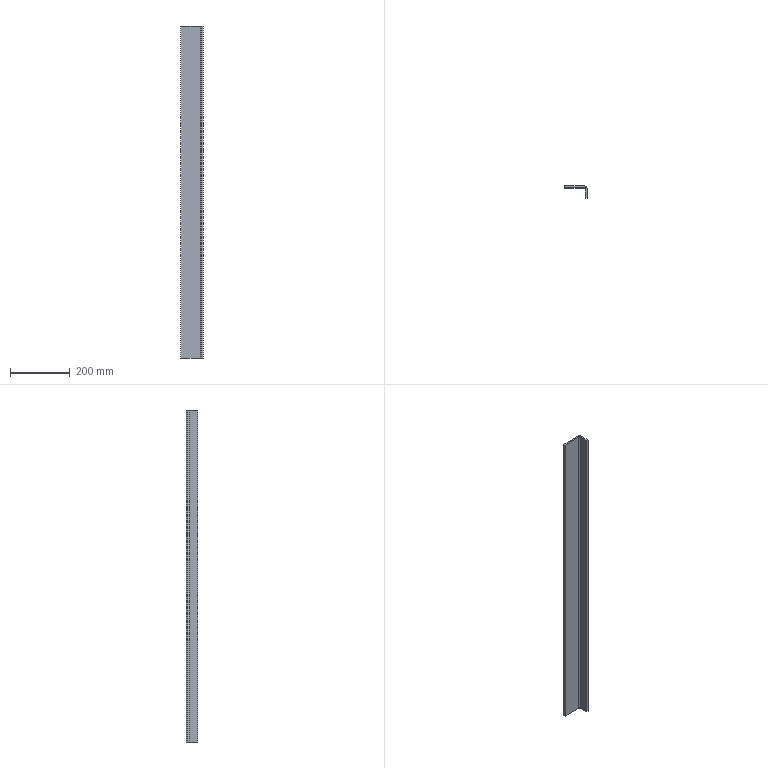Part | SolidWorks | features Extrusion 1 | 1 solid | 10 faces | box 75 x 40 x 1110 mm | volume 705931 mm3 | plane 8 | cylinder 2 | commonest cylinder face diameters 8 x1 20 x1
STEP:
#1=CARTESIAN_POINT('',(75.,-10.,0.));
#2=VERTEX_POINT('',#1);
#3=CARTESIAN_POINT('',(75.,-40.,0.));
#4=VERTEX_POINT('',#3);
#5=CARTESIAN_POINT('',(75.,-10.,0.));
#6=DIRECTION('',(0.,-1.,0.));
#7=VECTOR('',#6,1000.);
#8=LINE('',#5,#7);
#9=EDGE_CURVE('',#2,#4,#8,.T.);
#10=ORIENTED_EDGE('',*,*,#9,.F.);
#11=CARTESIAN_POINT('',(75.,-10.,1110.));
#12=VERTEX_POINT('',#11);
#13=CARTESIAN_POINT('',(75.,-10.,1110.));
#14=DIRECTION('',(0.,0.,-1.));
#15=VECTOR('',#14,1000.);
#16=LINE('',#13,#15);
#17=EDGE_CURVE('',#12,#2,#16,.T.);
#18=ORIENTED_EDGE('',*,*,#17,.F.);
#19=CARTESIAN_POINT('',(75.,-40.,1110.));
#20=VERTEX_POINT('',#19);
#21=CARTESIAN_POINT('',(75.,-10.,1110.));
#22=DIRECTION('',(0.,-1.,0.));
#23=VECTOR('',#22,1000.);
#24=LINE('',#21,#23);
#25=EDGE_CURVE('',#12,#20,#24,.T.);
#26=ORIENTED_EDGE('',*,*,#25,.T.);
#27=CARTESIAN_POINT('',(75.,-40.,1110.));
#28=DIRECTION('',(0.,0.,-1.));
#29=VECTOR('',#28,1000.);
#30=LINE('',#27,#29);
#31=EDGE_CURVE('',#20,#4,#30,.T.);
#32=ORIENTED_EDGE('',*,*,#31,.T.);
#33=EDGE_LOOP('',(#10,#18,#26,#32));
#34=FACE_OUTER_BOUND('',#33,.T.);
#35=CARTESIAN_POINT('',(75.,-10.,1110.));
#36=DIRECTION('',(1.,0.,0.));
#37=DIRECTION('',(0.,0.,-1.));
#38=AXIS2_PLACEMENT_3D('',#35,#36,#37);
#39=PLANE('',#38);
#40=ADVANCED_FACE('',(#34),#39,.T.);
#41=CARTESIAN_POINT('',(65.,0.,0.));
#42=VERTEX_POINT('',#41);
#43=CARTESIAN_POINT('',(65.,-10.,0.));
#44=DIRECTION('',(0.,0.,-1.));
#45=DIRECTION('',(-1.,0.,0.));
#46=AXIS2_PLACEMENT_3D('',#43,#44,#45);
#47=CIRCLE('',#46,10.);
#48=EDGE_CURVE('',#42,#2,#47,.T.);
#49=ORIENTED_EDGE('',*,*,#48,.F.);
#50=CARTESIAN_POINT('',(65.,0.,1110.));
#51=VERTEX_POINT('',#50);
#52=CARTESIAN_POINT('',(65.,0.,1110.));
#53=DIRECTION('',(0.,0.,-1.));
#54=VECTOR('',#53,1000.);
#55=LINE('',#52,#54);
#56=EDGE_CURVE('',#51,#42,#55,.T.);
#57=ORIENTED_EDGE('',*,*,#56,.F.);
#58=CARTESIAN_POINT('',(65.,-10.,1110.));
#59=DIRECTION('',(0.,0.,-1.));
#60=DIRECTION('',(-1.,0.,0.));
#61=AXIS2_PLACEMENT_3D('',#58,#59,#60);
#62=CIRCLE('',#61,10.);
#63=EDGE_CURVE('',#51,#12,#62,.T.);
#64=ORIENTED_EDGE('',*,*,#63,.T.);
#65=ORIENTED_EDGE('',*,*,#17,.T.);
#66=EDGE_LOOP('',(#49,#57,#64,#65));
#67=FACE_OUTER_BOUND('',#66,.T.);
#68=CARTESIAN_POINT('',(65.,-10.,1110.));
#69=DIRECTION('',(0.,0.,-1.));
#70=DIRECTION('',(-1.,0.,0.));
#71=AXIS2_PLACEMENT_3D('',#68,#69,#70);
#72=CYLINDRICAL_SURFACE('',#71,10.);
#73=ADVANCED_FACE('',(#67),#72,.T.);
#74=CARTESIAN_POINT('',(0.,0.,0.));
#75=VERTEX_POINT('',#74);
#76=CARTESIAN_POINT('',(0.,0.,0.));
#77=DIRECTION('',(1.,0.,0.));
#78=VECTOR('',#77,1000.);
#79=LINE('',#76,#78);
#80=EDGE_CURVE('',#75,#42,#79,.T.);
#81=ORIENTED_EDGE('',*,*,#80,.F.);
#82=CARTESIAN_POINT('',(0.,0.,1110.));
#83=VERTEX_POINT('',#82);
#84=CARTESIAN_POINT('',(0.,0.,1110.));
#85=DIRECTION('',(0.,0.,-1.));
#86=VECTOR('',#85,1000.);
#87=LINE('',#84,#86);
#88=EDGE_CURVE('',#83,#75,#87,.T.);
#89=ORIENTED_EDGE('',*,*,#88,.F.);
#90=CARTESIAN_POINT('',(0.,0.,1110.));
#91=DIRECTION('',(1.,0.,0.));
#92=VECTOR('',#91,1000.);
#93=LINE('',#90,#92);
#94=EDGE_CURVE('',#83,#51,#93,.T.);
#95=ORIENTED_EDGE('',*,*,#94,.T.);
#96=ORIENTED_EDGE('',*,*,#56,.T.);
#97=EDGE_LOOP('',(#81,#89,#95,#96));
#98=FACE_OUTER_BOUND('',#97,.T.);
#99=CARTESIAN_POINT('',(0.,0.,1110.));
#100=DIRECTION('',(0.,1.,0.));
#101=DIRECTION('',(0.,0.,1.));
#102=AXIS2_PLACEMENT_3D('',#99,#100,#101);
#103=PLANE('',#102);
#104=ADVANCED_FACE('',(#98),#103,.T.);
#105=CARTESIAN_POINT('',(0.,-6.,0.));
#106=VERTEX_POINT('',#105);
#107=CARTESIAN_POINT('',(0.,0.,0.));
#108=DIRECTION('',(0.,-1.,0.));
#109=VECTOR('',#108,1000.);
#110=LINE('',#107,#109);
#111=EDGE_CURVE('',#75,#106,#110,.T.);
#112=ORIENTED_EDGE('',*,*,#111,.T.);
#113=CARTESIAN_POINT('',(0.,-6.,1110.));
#114=VERTEX_POINT('',#113);
#115=CARTESIAN_POINT('',(0.,-6.,1110.));
#116=DIRECTION('',(0.,0.,-1.));
#117=VECTOR('',#116,1000.);
#118=LINE('',#115,#117);
#119=EDGE_CURVE('',#114,#106,#118,.T.);
#120=ORIENTED_EDGE('',*,*,#119,.F.);
#121=CARTESIAN_POINT('',(0.,0.,1110.));
#122=DIRECTION('',(0.,-1.,0.));
#123=VECTOR('',#122,1000.);
#124=LINE('',#121,#123);
#125=EDGE_CURVE('',#83,#114,#124,.T.);
#126=ORIENTED_EDGE('',*,*,#125,.F.);
#127=ORIENTED_EDGE('',*,*,#88,.T.);
#128=EDGE_LOOP('',(#112,#120,#126,#127));
#129=FACE_OUTER_BOUND('',#128,.T.);
#130=CARTESIAN_POINT('',(0.,0.,1110.));
#131=DIRECTION('',(1.,0.,0.));
#132=DIRECTION('',(0.,0.,-1.));
#133=AXIS2_PLACEMENT_3D('',#130,#131,#132);
#134=PLANE('',#133);
#135=ADVANCED_FACE('',(#129),#134,.F.);
#136=CARTESIAN_POINT('',(65.,-6.,0.));
#137=VERTEX_POINT('',#136);
#138=CARTESIAN_POINT('',(0.,-6.,0.));
#139=DIRECTION('',(1.,0.,0.));
#140=VECTOR('',#139,1000.);
#141=LINE('',#138,#140);
#142=EDGE_CURVE('',#106,#137,#141,.T.);
#143=ORIENTED_EDGE('',*,*,#142,.T.);
#144=CARTESIAN_POINT('',(65.,-6.,1110.));
#145=VERTEX_POINT('',#144);
#146=CARTESIAN_POINT('',(65.,-6.,1110.));
#147=DIRECTION('',(0.,0.,-1.));
#148=VECTOR('',#147,1000.);
#149=LINE('',#146,#148);
#150=EDGE_CURVE('',#145,#137,#149,.T.);
#151=ORIENTED_EDGE('',*,*,#150,.F.);
#152=CARTESIAN_POINT('',(0.,-6.,1110.));
#153=DIRECTION('',(1.,0.,0.));
#154=VECTOR('',#153,1000.);
#155=LINE('',#152,#154);
#156=EDGE_CURVE('',#114,#145,#155,.T.);
#157=ORIENTED_EDGE('',*,*,#156,.F.);
#158=ORIENTED_EDGE('',*,*,#119,.T.);
#159=EDGE_LOOP('',(#143,#151,#157,#158));
#160=FACE_OUTER_BOUND('',#159,.T.);
#161=CARTESIAN_POINT('',(0.,-6.,1110.));
#162=DIRECTION('',(0.,1.,0.));
#163=DIRECTION('',(0.,0.,1.));
#164=AXIS2_PLACEMENT_3D('',#161,#162,#163);
#165=PLANE('',#164);
#166=ADVANCED_FACE('',(#160),#165,.F.);
#167=CARTESIAN_POINT('',(69.,-10.,0.));
#168=VERTEX_POINT('',#167);
#169=CARTESIAN_POINT('',(65.,-10.,0.));
#170=DIRECTION('',(0.,0.,-1.));
#171=DIRECTION('',(-1.,0.,0.));
#172=AXIS2_PLACEMENT_3D('',#169,#170,#171);
#173=CIRCLE('',#172,4.);
#174=EDGE_CURVE('',#137,#168,#173,.T.);
#175=ORIENTED_EDGE('',*,*,#174,.T.);
#176=CARTESIAN_POINT('',(69.,-10.,1110.));
#177=VERTEX_POINT('',#176);
#178=CARTESIAN_POINT('',(69.,-10.,1110.));
#179=DIRECTION('',(0.,0.,-1.));
#180=VECTOR('',#179,1000.);
#181=LINE('',#178,#180);
#182=EDGE_CURVE('',#177,#168,#181,.T.);
#183=ORIENTED_EDGE('',*,*,#182,.F.);
#184=CARTESIAN_POINT('',(65.,-10.,1110.));
#185=DIRECTION('',(0.,0.,-1.));
#186=DIRECTION('',(-1.,0.,0.));
#187=AXIS2_PLACEMENT_3D('',#184,#185,#186);
#188=CIRCLE('',#187,4.);
#189=EDGE_CURVE('',#145,#177,#188,.T.);
#190=ORIENTED_EDGE('',*,*,#189,.F.);
#191=ORIENTED_EDGE('',*,*,#150,.T.);
#192=EDGE_LOOP('',(#175,#183,#190,#191));
#193=FACE_OUTER_BOUND('',#192,.T.);
#194=CARTESIAN_POINT('',(65.,-10.,1110.));
#195=DIRECTION('',(0.,0.,-1.));
#196=DIRECTION('',(-1.,0.,0.));
#197=AXIS2_PLACEMENT_3D('',#194,#195,#196);
#198=CYLINDRICAL_SURFACE('',#197,4.);
#199=ADVANCED_FACE('',(#193),#198,.F.);
#200=CARTESIAN_POINT('',(69.,-40.,0.));
#201=VERTEX_POINT('',#200);
#202=CARTESIAN_POINT('',(69.,-10.,0.));
#203=DIRECTION('',(0.,-1.,0.));
#204=VECTOR('',#203,1000.);
#205=LINE('',#202,#204);
#206=EDGE_CURVE('',#168,#201,#205,.T.);
#207=ORIENTED_EDGE('',*,*,#206,.T.);
#208=CARTESIAN_POINT('',(69.,-40.,1110.));
#209=VERTEX_POINT('',#208);
#210=CARTESIAN_POINT('',(69.,-40.,1110.));
#211=DIRECTION('',(0.,0.,-1.));
#212=VECTOR('',#211,1000.);
#213=LINE('',#210,#212);
#214=EDGE_CURVE('',#209,#201,#213,.T.);
#215=ORIENTED_EDGE('',*,*,#214,.F.);
#216=CARTESIAN_POINT('',(69.,-10.,1110.));
#217=DIRECTION('',(0.,-1.,0.));
#218=VECTOR('',#217,1000.);
#219=LINE('',#216,#218);
#220=EDGE_CURVE('',#177,#209,#219,.T.);
#221=ORIENTED_EDGE('',*,*,#220,.F.);
#222=ORIENTED_EDGE('',*,*,#182,.T.);
#223=EDGE_LOOP('',(#207,#215,#221,#222));
#224=FACE_OUTER_BOUND('',#223,.T.);
#225=CARTESIAN_POINT('',(69.,-10.,1110.));
#226=DIRECTION('',(1.,0.,0.));
#227=DIRECTION('',(0.,1.,0.));
#228=AXIS2_PLACEMENT_3D('',#225,#226,#227);
#229=PLANE('',#228);
#230=ADVANCED_FACE('',(#224),#229,.F.);
#231=CARTESIAN_POINT('',(75.,-40.,0.));
#232=DIRECTION('',(-1.,0.,0.));
#233=VECTOR('',#232,1000.);
#234=LINE('',#231,#233);
#235=EDGE_CURVE('',#4,#201,#234,.T.);
#236=ORIENTED_EDGE('',*,*,#235,.F.);
#237=ORIENTED_EDGE('',*,*,#31,.F.);
#238=CARTESIAN_POINT('',(75.,-40.,1110.));
#239=DIRECTION('',(-1.,0.,0.));
#240=VECTOR('',#239,1000.);
#241=LINE('',#238,#240);
#242=EDGE_CURVE('',#20,#209,#241,.T.);
#243=ORIENTED_EDGE('',*,*,#242,.T.);
#244=ORIENTED_EDGE('',*,*,#214,.T.);
#245=EDGE_LOOP('',(#236,#237,#243,#244));
#246=FACE_OUTER_BOUND('',#245,.T.);
#247=CARTESIAN_POINT('',(75.,-40.,1110.));
#248=DIRECTION('',(0.,-1.,0.));
#249=DIRECTION('',(0.,0.,-1.));
#250=AXIS2_PLACEMENT_3D('',#247,#248,#249);
#251=PLANE('',#250);
#252=ADVANCED_FACE('',(#246),#251,.T.);
#253=ORIENTED_EDGE('',*,*,#25,.F.);
#254=ORIENTED_EDGE('',*,*,#63,.F.);
#255=ORIENTED_EDGE('',*,*,#94,.F.);
#256=ORIENTED_EDGE('',*,*,#125,.T.);
#257=ORIENTED_EDGE('',*,*,#156,.T.);
#258=ORIENTED_EDGE('',*,*,#189,.T.);
#259=ORIENTED_EDGE('',*,*,#220,.T.);
#260=ORIENTED_EDGE('',*,*,#242,.F.);
#261=EDGE_LOOP('',(#253,#254,#255,#256,#257,#258,#259,#260));
#262=FACE_OUTER_BOUND('',#261,.T.);
#263=CARTESIAN_POINT('',(65.,-10.,1110.));
#264=DIRECTION('',(0.,0.,-1.));
#265=DIRECTION('',(-1.,0.,0.));
#266=AXIS2_PLACEMENT_3D('',#263,#264,#265);
#267=PLANE('',#266);
#268=ADVANCED_FACE('',(#262),#267,.F.);
#269=ORIENTED_EDGE('',*,*,#9,.T.);
#270=ORIENTED_EDGE('',*,*,#235,.T.);
#271=ORIENTED_EDGE('',*,*,#206,.F.);
#272=ORIENTED_EDGE('',*,*,#174,.F.);
#273=ORIENTED_EDGE('',*,*,#142,.F.);
#274=ORIENTED_EDGE('',*,*,#111,.F.);
#275=ORIENTED_EDGE('',*,*,#80,.T.);
#276=ORIENTED_EDGE('',*,*,#48,.T.);
#277=EDGE_LOOP('',(#269,#270,#271,#272,#273,#274,#275,#276));
#278=FACE_OUTER_BOUND('',#277,.T.);
#279=CARTESIAN_POINT('',(65.,-10.,0.));
#280=DIRECTION('',(0.,0.,-1.));
#281=DIRECTION('',(-1.,0.,0.));
#282=AXIS2_PLACEMENT_3D('',#279,#280,#281);
#283=PLANE('',#282);
#284=ADVANCED_FACE('',(#278),#283,.T.);
#285=CLOSED_SHELL('',(#40,#73,#104,#135,#166,#199,#230,#252,#268,#284));
#286=MANIFOLD_SOLID_BREP('',#285);
#287=CARTESIAN_POINT('',(0.,0.,0.));
#288=DIRECTION('',(0.,0.,1.));
#289=DIRECTION('',(1.,0.,0.));
#290=AXIS2_PLACEMENT_3D('',#287,#288,#289);
#291=(LENGTH_UNIT()NAMED_UNIT(*)SI_UNIT(.MILLI.,.METRE.));
#292=UNCERTAINTY_MEASURE_WITH_UNIT(LENGTH_MEASURE(0.00001),#291,'','');
#293=(NAMED_UNIT(*)PLANE_ANGLE_UNIT()SI_UNIT($,.RADIAN.));
#294=(NAMED_UNIT(*)SI_UNIT($,.STERADIAN.)SOLID_ANGLE_UNIT());
#295=(GEOMETRIC_REPRESENTATION_CONTEXT(3)GLOBAL_UNCERTAINTY_ASSIGNED_CONTEXT((#292))GLOBAL_UNIT_ASSIGNED_CONTEXT((#291,#293,#294))REPRESENTATION_CONTEXT('',''));
#296=ADVANCED_BREP_SHAPE_REPRESENTATION('',(#286,#290),#295);